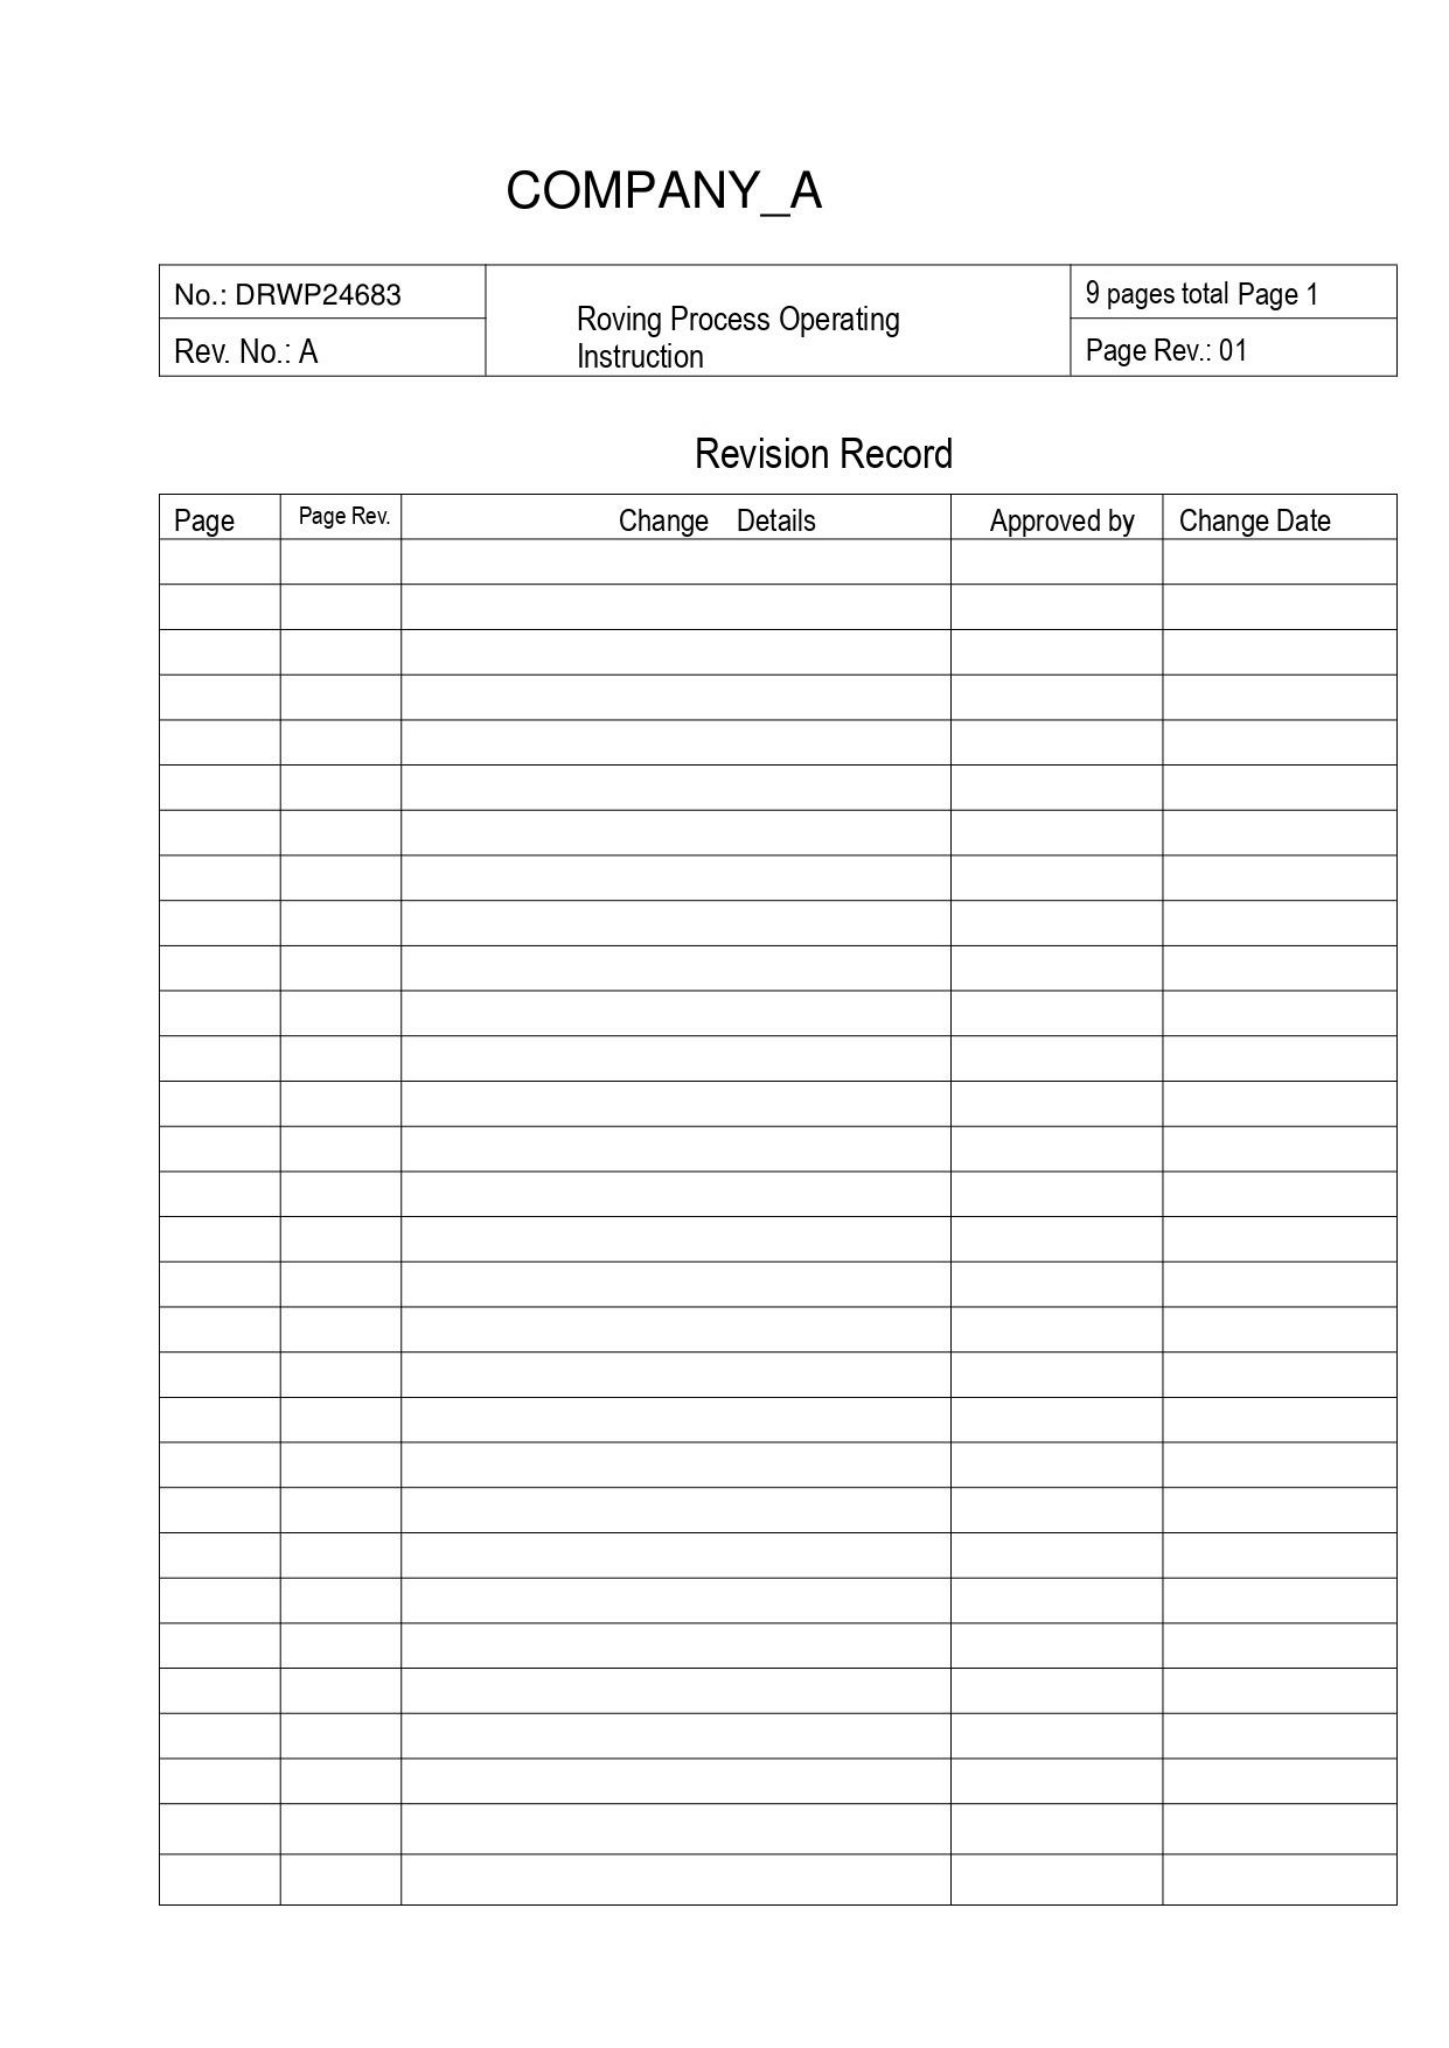COMPANY_A

| No.: DRWP24683 | Roving Process Operating Instruction | 9 pages total Page 1 |
|---|---|---|
| Rev. No.: A | | Page Rev.: 01 |

Revision Record

| Page | Page Rev. | Change Details | Approved by | Change Date |
|---|---|---|---|---|
| | | | | |
| | | | | |
| | | | | |
| | | | | |
| | | | | |
| | | | | |
| | | | | |
| | | | | |
| | | | | |
| | | | | |
| | | | | |
| | | | | |
| | | | | |
| | | | | |
| | | | | |
| | | | | |
| | | | | |
| | | | | |
| | | | | |
| | | | | |
| | | | | |
| | | | | |
| | | | | |
| | | | | |
| | | | | |
| | | | | |
| | | | | |
| | | | | |
| | | | | |
| | | | | |
| | | | | |
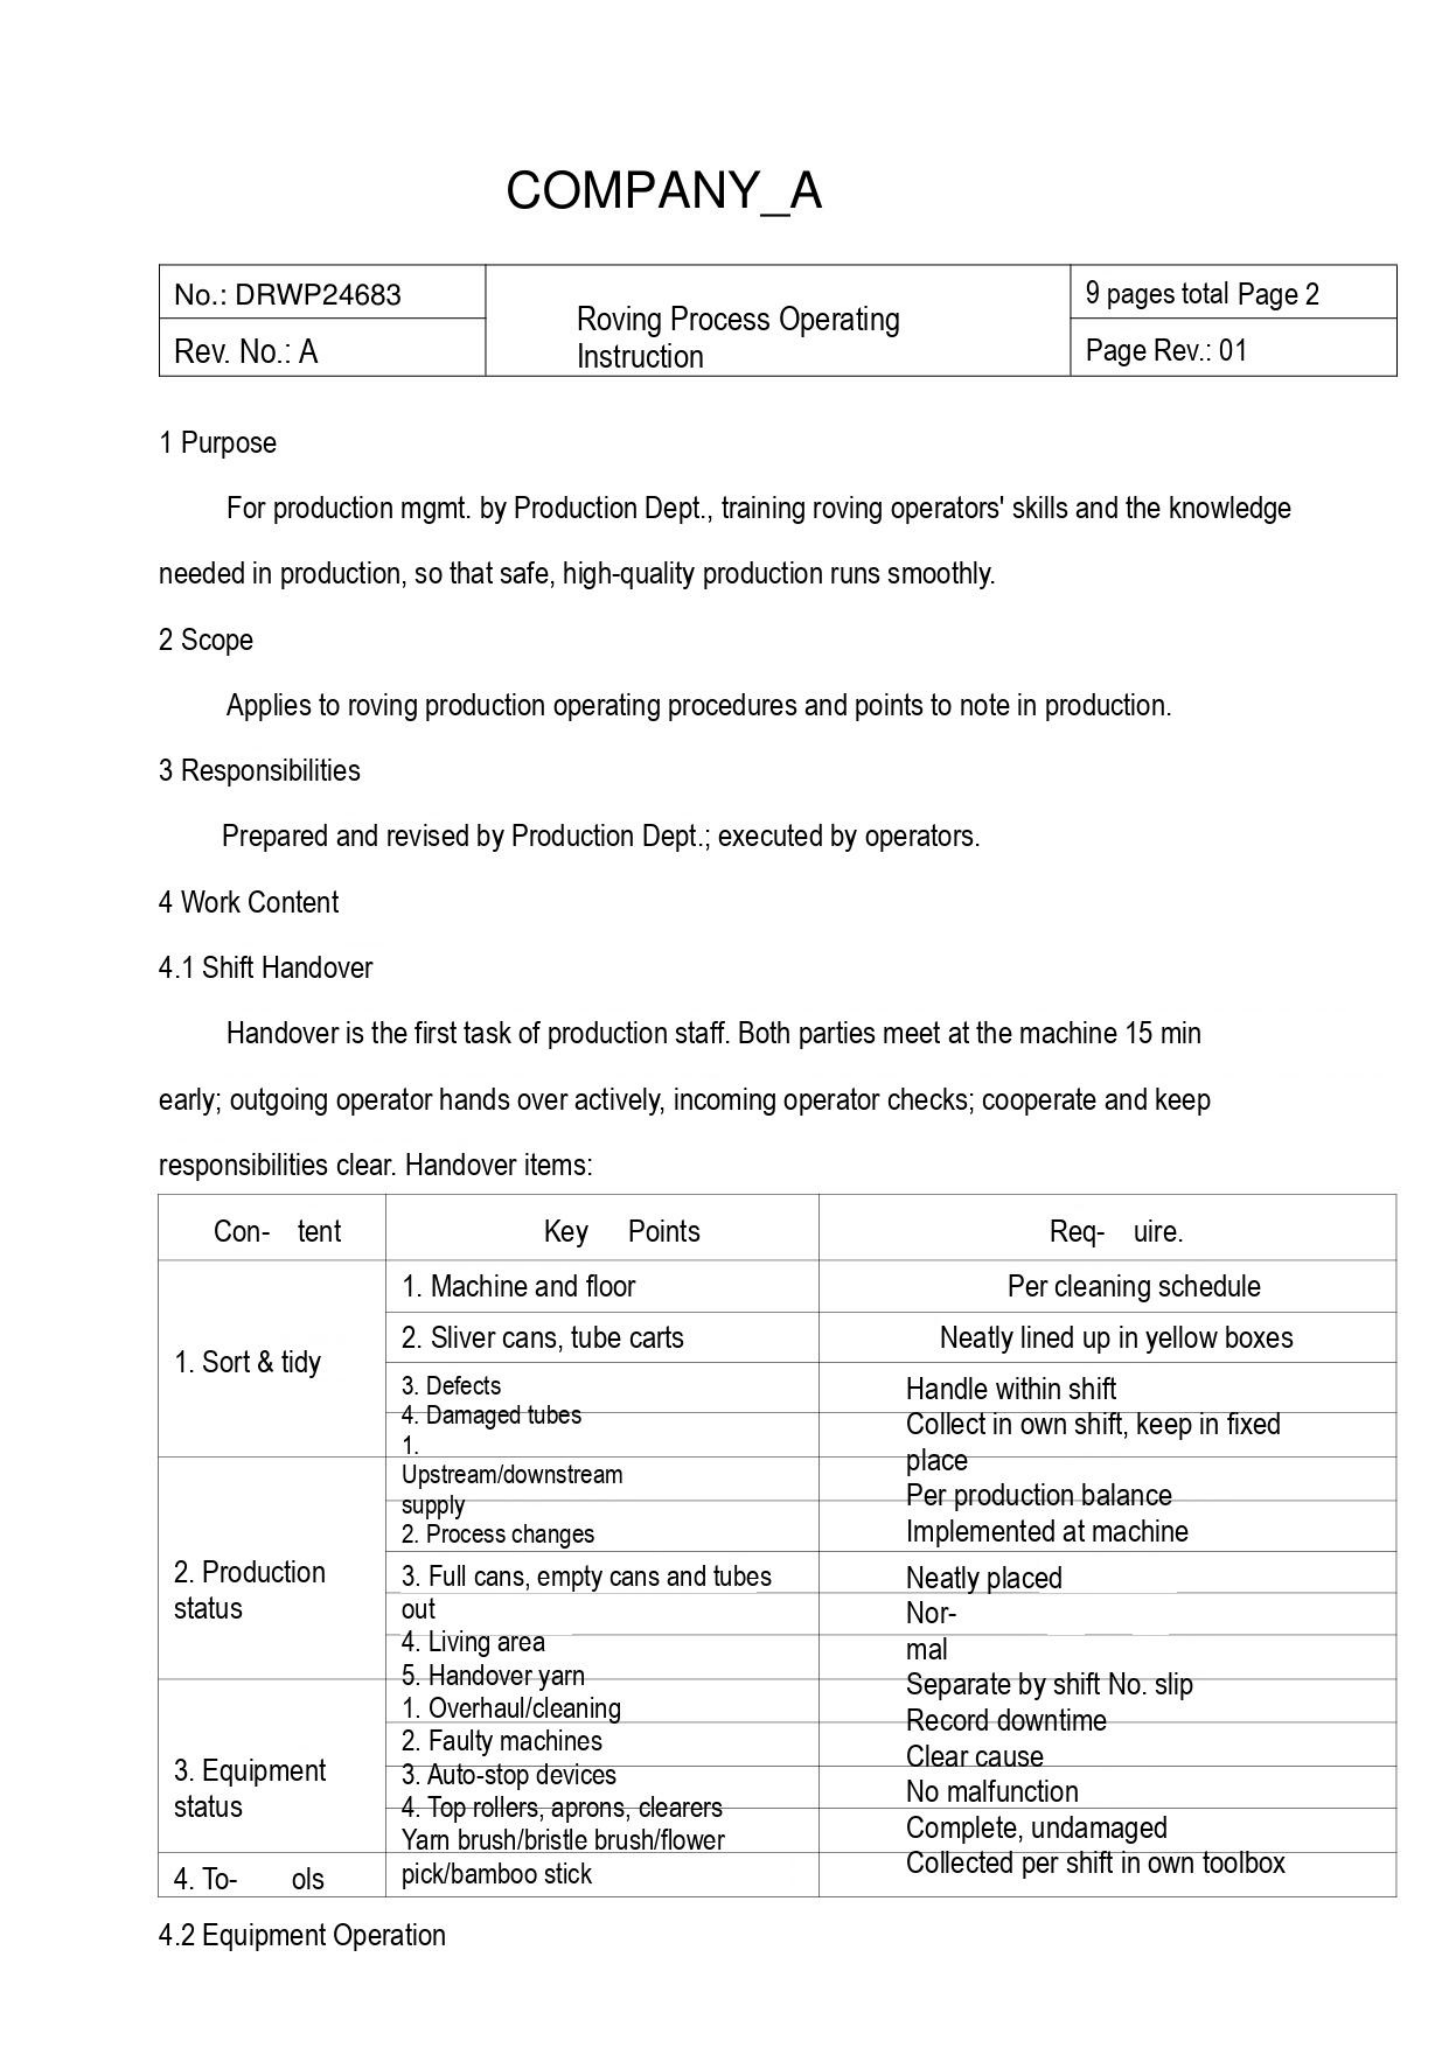# COMPANY_A

| No.: DRWP24683 | Roving Process Operating Instruction | 9 pages total Page 2 |
|---|---|---|
| Rev. No.: A | | Page Rev.: 01 |

1 Purpose

For production mgmt. by Production Dept., training roving operators' skills and the knowledge needed in production, so that safe, high-quality production runs smoothly.

2 Scope

Applies to roving production operating procedures and points to note in production.

3 Responsibilities

Prepared and revised by Production Dept.; executed by operators.

4 Work Content

4.1 Shift Handover

Handover is the first task of production staff. Both parties meet at the machine 15 min early; outgoing operator hands over actively, incoming operator checks; cooperate and keep responsibilities clear. Handover items:

| Con- tent | Key Points | Req- uire. |
|---|---|---|
| 1. Sort & tidy | 1. Machine and floor | Per cleaning schedule |
| | 2. Sliver cans, tube carts | Neatly lined up in yellow boxes |
| | 3. Defects | Handle within shift |
| | 4. Damaged tubes | Collect in own shift, keep in fixed place |
| 2. Production status | 1. Upstream/downstream supply | Per production balance |
| | 2. Process changes | Implemented at machine |
| | 3. Full cans, empty cans and tubes out | Neatly placed |
| | 4. Living area | Nor- mal |
| | 5. Handover yarn | Separate by shift No. slip |
| 3. Equipment status | 1. Overhaul/cleaning | Record downtime |
| | 2. Faulty machines | Clear cause |
| | 3. Auto-stop devices | No malfunction |
| | 4. Top rollers, aprons, clearers | Complete, undamaged |
| 4. To- ols | Yarn brush/bristle brush/flower pick/bamboo stick | Collected per shift in own toolbox |

4.2 Equipment Operation
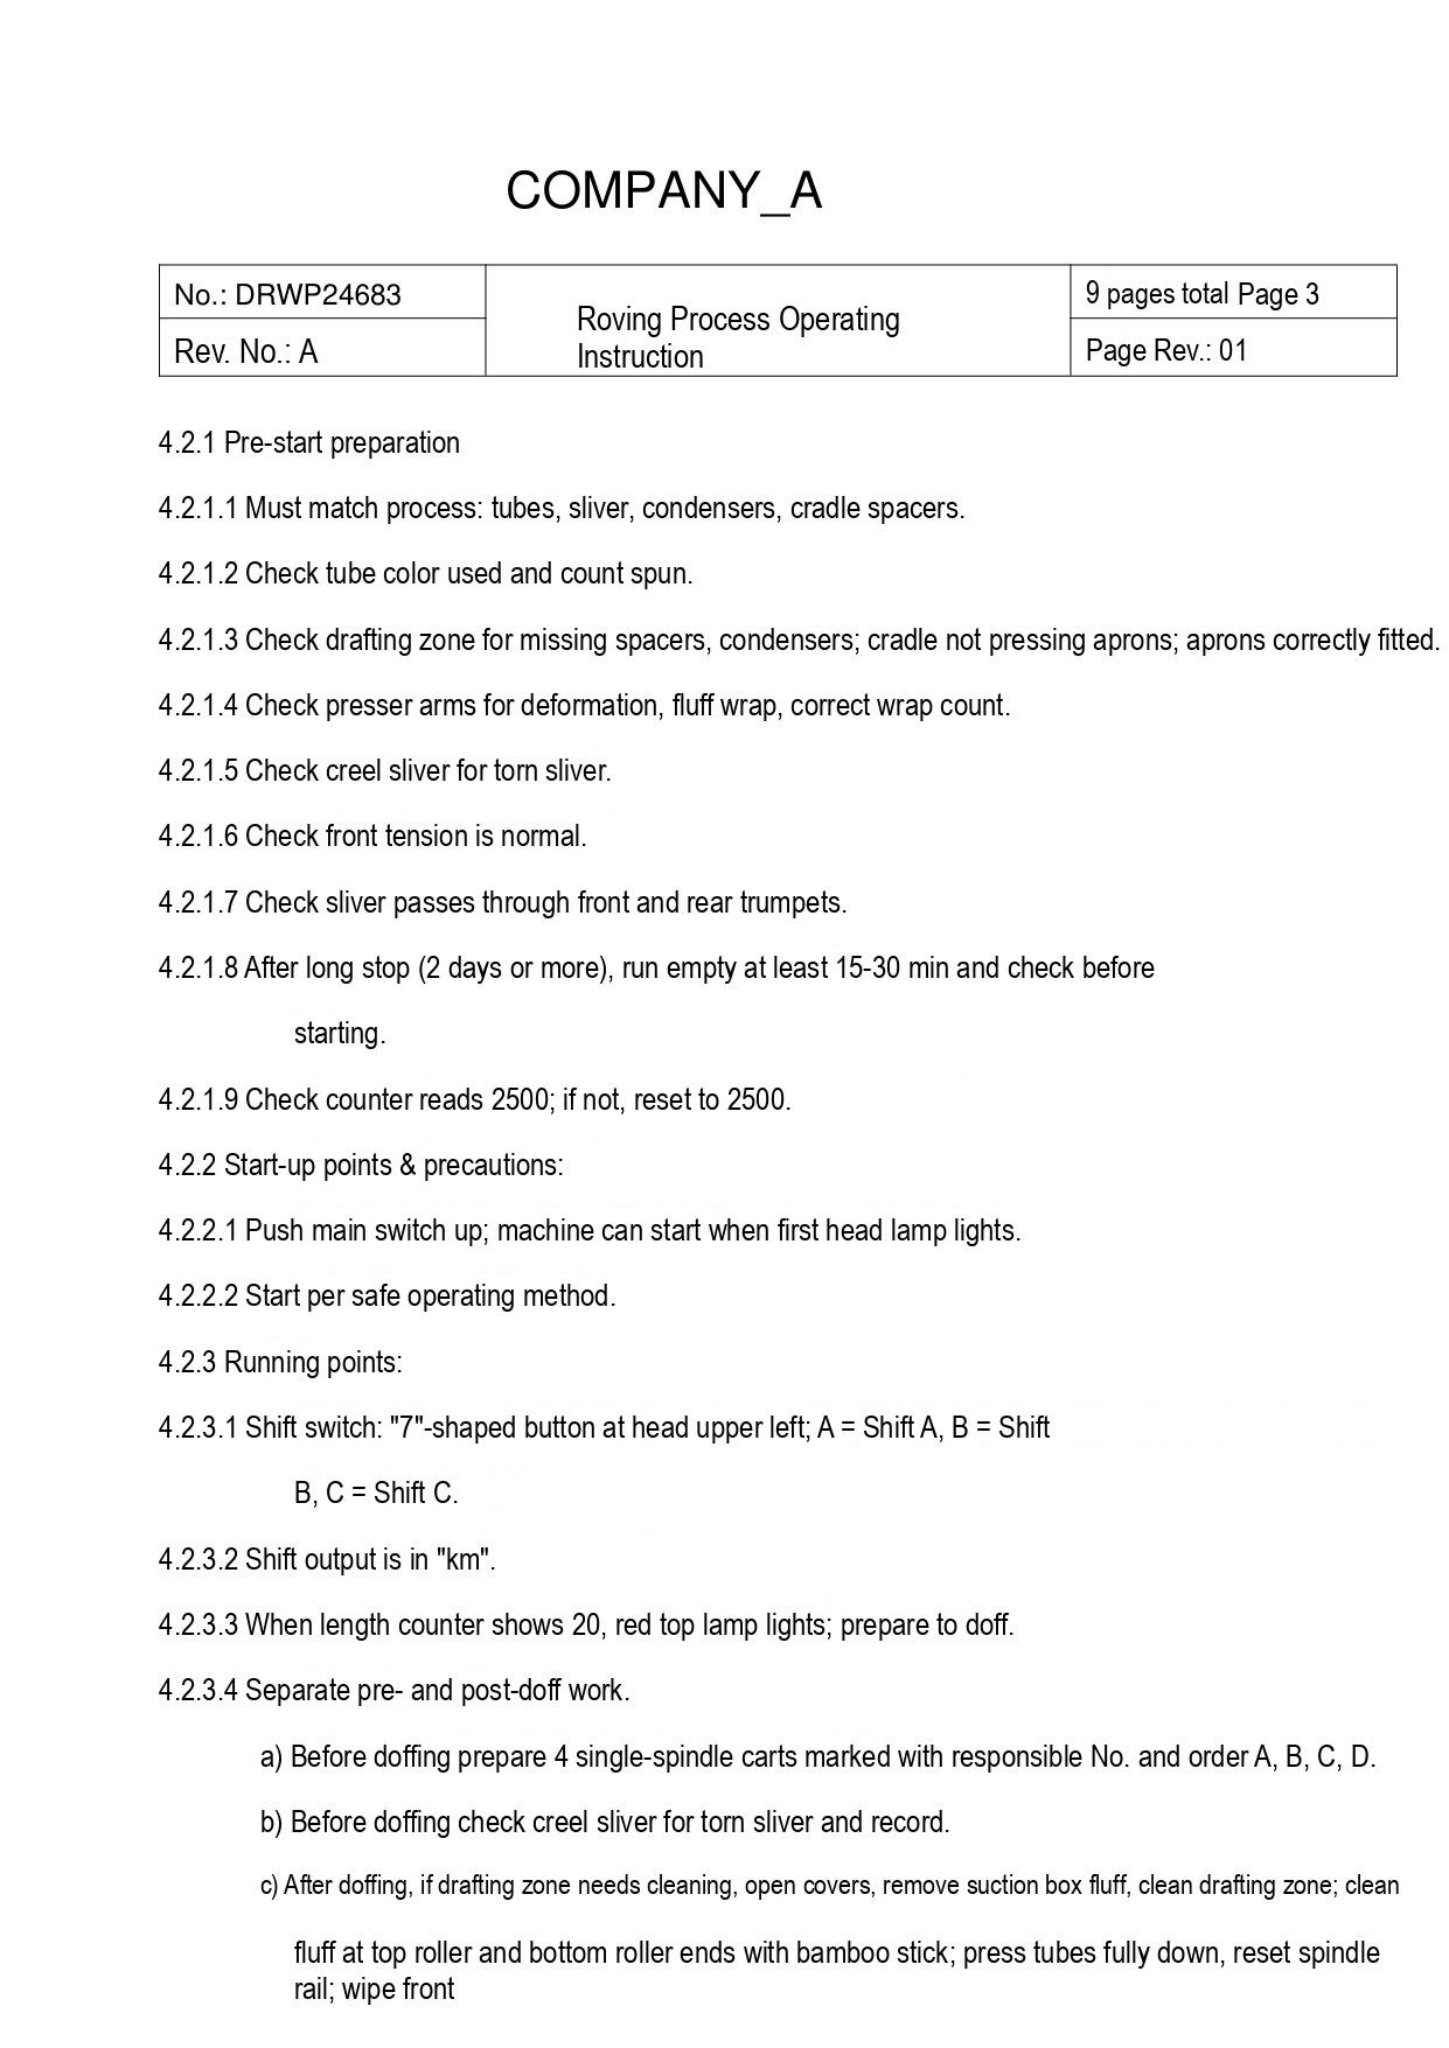COMPANY_A

| No.: DRWP24683 | Roving Process Operating Instruction | 9 pages total Page 3 |
|---|---|---|
| Rev. No.: A | | Page Rev.: 01 |

4.2.1 Pre-start preparation

4.2.1.1 Must match process: tubes, sliver, condensers, cradle spacers.

4.2.1.2 Check tube color used and count spun.

4.2.1.3 Check drafting zone for missing spacers, condensers; cradle not pressing aprons; aprons correctly fitted.

4.2.1.4 Check presser arms for deformation, fluff wrap, correct wrap count.

4.2.1.5 Check creel sliver for torn sliver.

4.2.1.6 Check front tension is normal.

4.2.1.7 Check sliver passes through front and rear trumpets.

4.2.1.8 After long stop (2 days or more), run empty at least 15-30 min and check before starting.

4.2.1.9 Check counter reads 2500; if not, reset to 2500.

4.2.2 Start-up points & precautions:

4.2.2.1 Push main switch up; machine can start when first head lamp lights.

4.2.2.2 Start per safe operating method.

4.2.3 Running points:

4.2.3.1 Shift switch: "7"-shaped button at head upper left; A = Shift A, B = Shift B, C = Shift C.

4.2.3.2 Shift output is in "km".

4.2.3.3 When length counter shows 20, red top lamp lights; prepare to doff.

4.2.3.4 Separate pre- and post-doff work.

a) Before doffing prepare 4 single-spindle carts marked with responsible No. and order A, B, C, D.

b) Before doffing check creel sliver for torn sliver and record.

c) After doffing, if drafting zone needs cleaning, open covers, remove suction box fluff, clean drafting zone; clean fluff at top roller and bottom roller ends with bamboo stick; press tubes fully down, reset spindle rail; wipe front
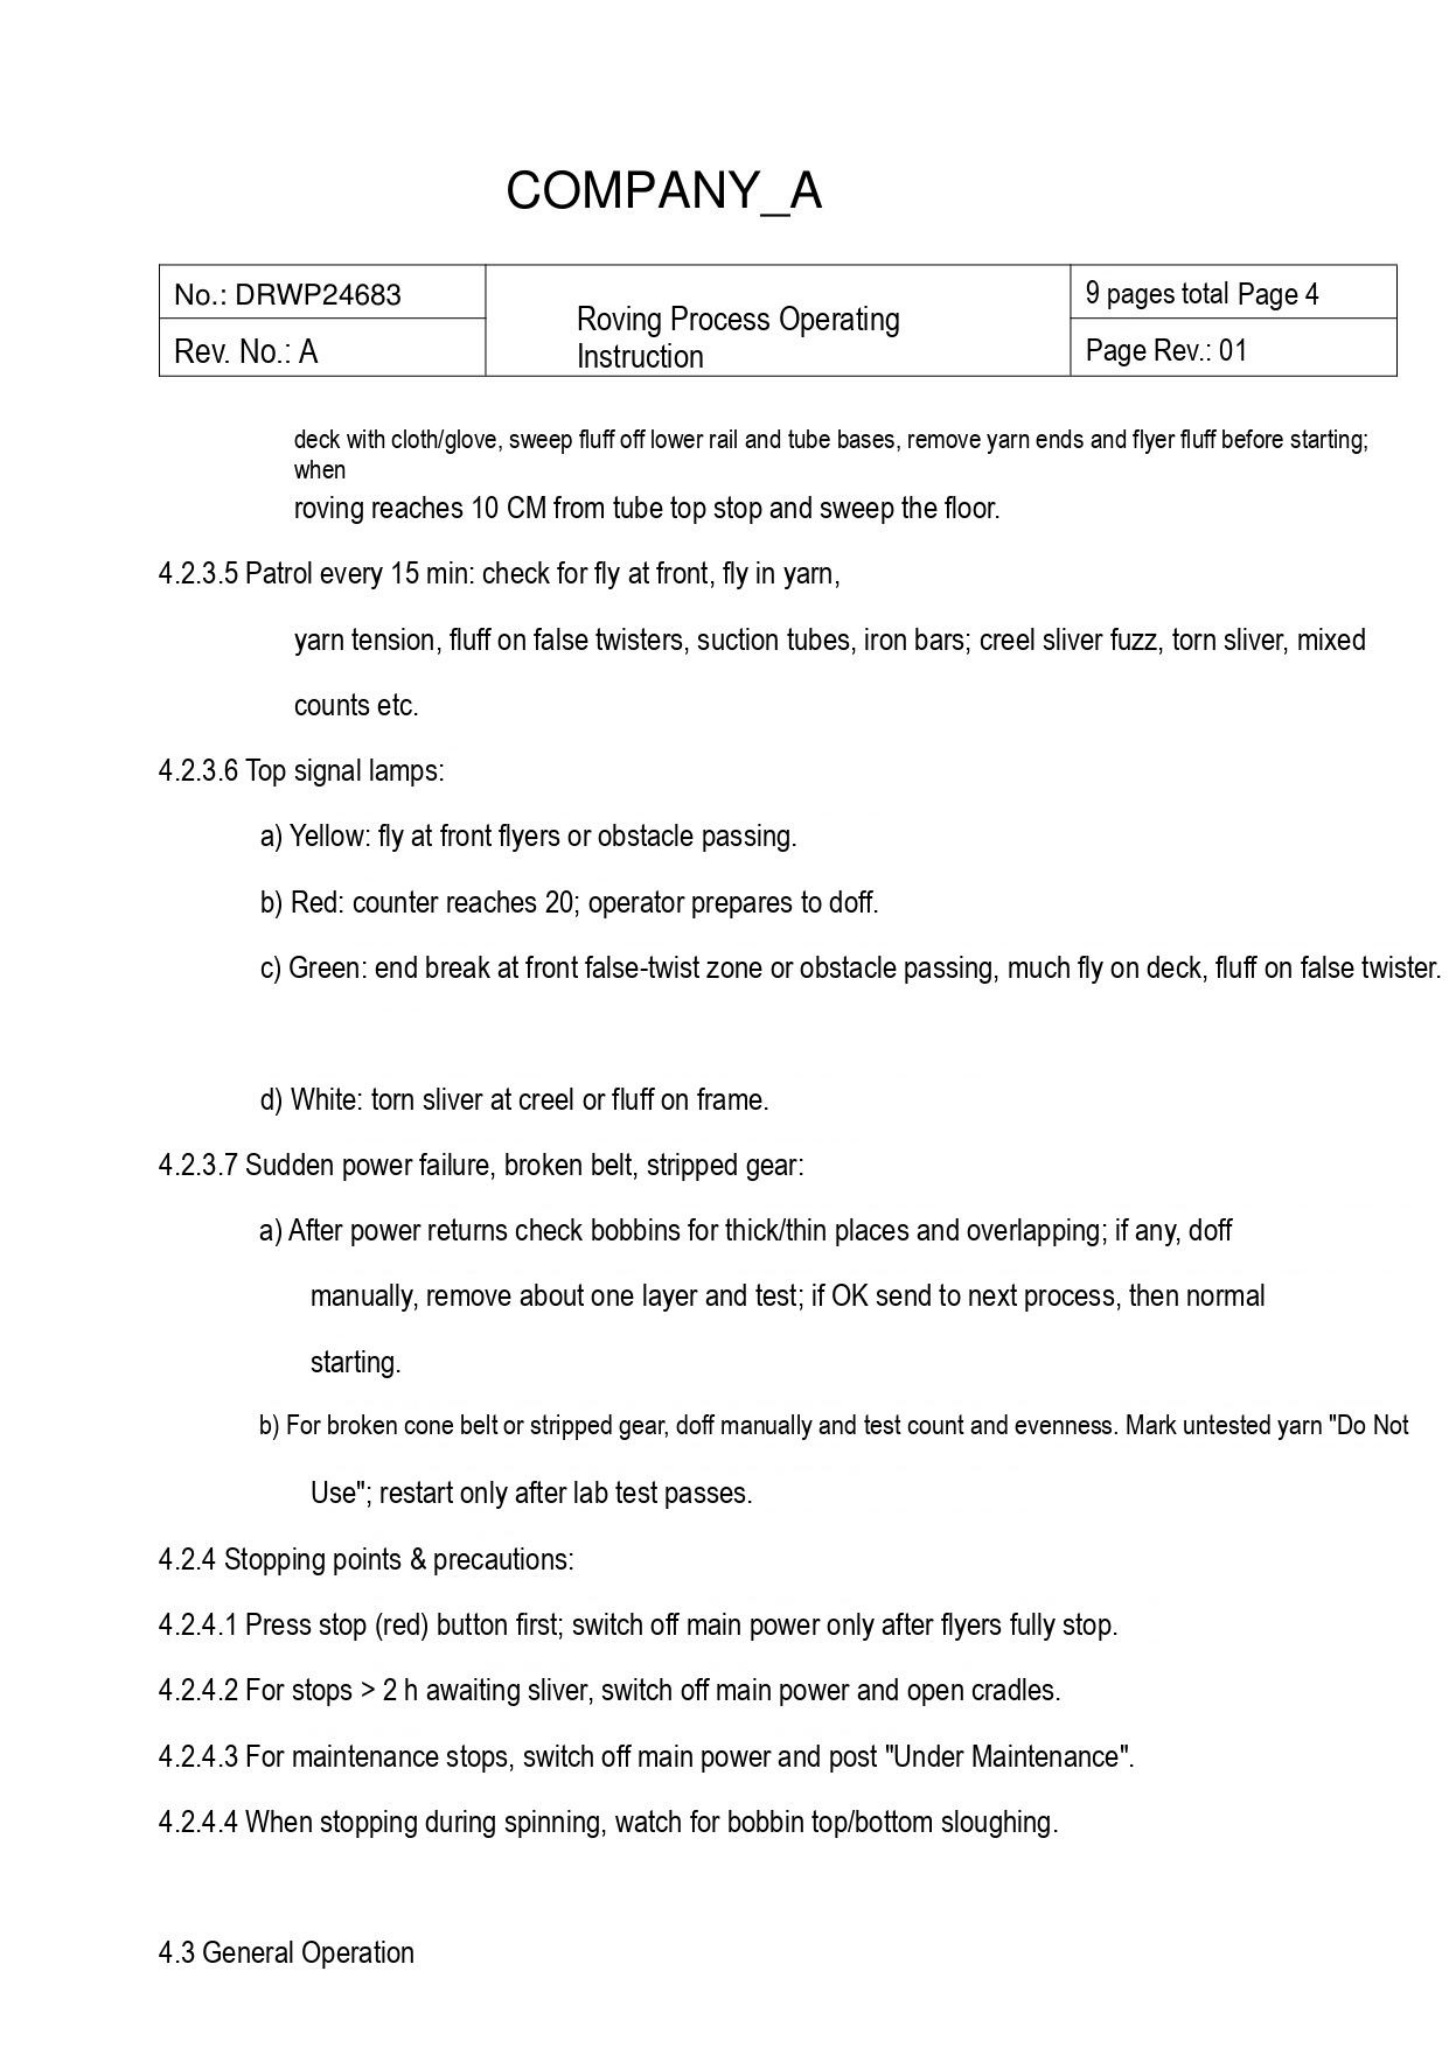COMPANY_A

| No.: DRWP24683 | Roving Process Operating Instruction | 9 pages total Page 4 |
|---|---|---|
| Rev. No.: A | | Page Rev.: 01 |

deck with cloth/glove, sweep fluff off lower rail and tube bases, remove yarn ends and flyer fluff before starting; when
roving reaches 10 CM from tube top stop and sweep the floor.

4.2.3.5 Patrol every 15 min: check for fly at front, fly in yarn,
yarn tension, fluff on false twisters, suction tubes, iron bars; creel sliver fuzz, torn sliver, mixed counts etc.

4.2.3.6 Top signal lamps:

a) Yellow: fly at front flyers or obstacle passing.

b) Red: counter reaches 20; operator prepares to doff.

c) Green: end break at front false-twist zone or obstacle passing, much fly on deck, fluff on false twister.

d) White: torn sliver at creel or fluff on frame.

4.2.3.7 Sudden power failure, broken belt, stripped gear:

a) After power returns check bobbins for thick/thin places and overlapping; if any, doff manually, remove about one layer and test; if OK send to next process, then normal starting.

b) For broken cone belt or stripped gear, doff manually and test count and evenness. Mark untested yarn "Do Not Use"; restart only after lab test passes.

4.2.4 Stopping points & precautions:

4.2.4.1 Press stop (red) button first; switch off main power only after flyers fully stop.

4.2.4.2 For stops > 2 h awaiting sliver, switch off main power and open cradles.

4.2.4.3 For maintenance stops, switch off main power and post "Under Maintenance".

4.2.4.4 When stopping during spinning, watch for bobbin top/bottom sloughing.

4.3 General Operation
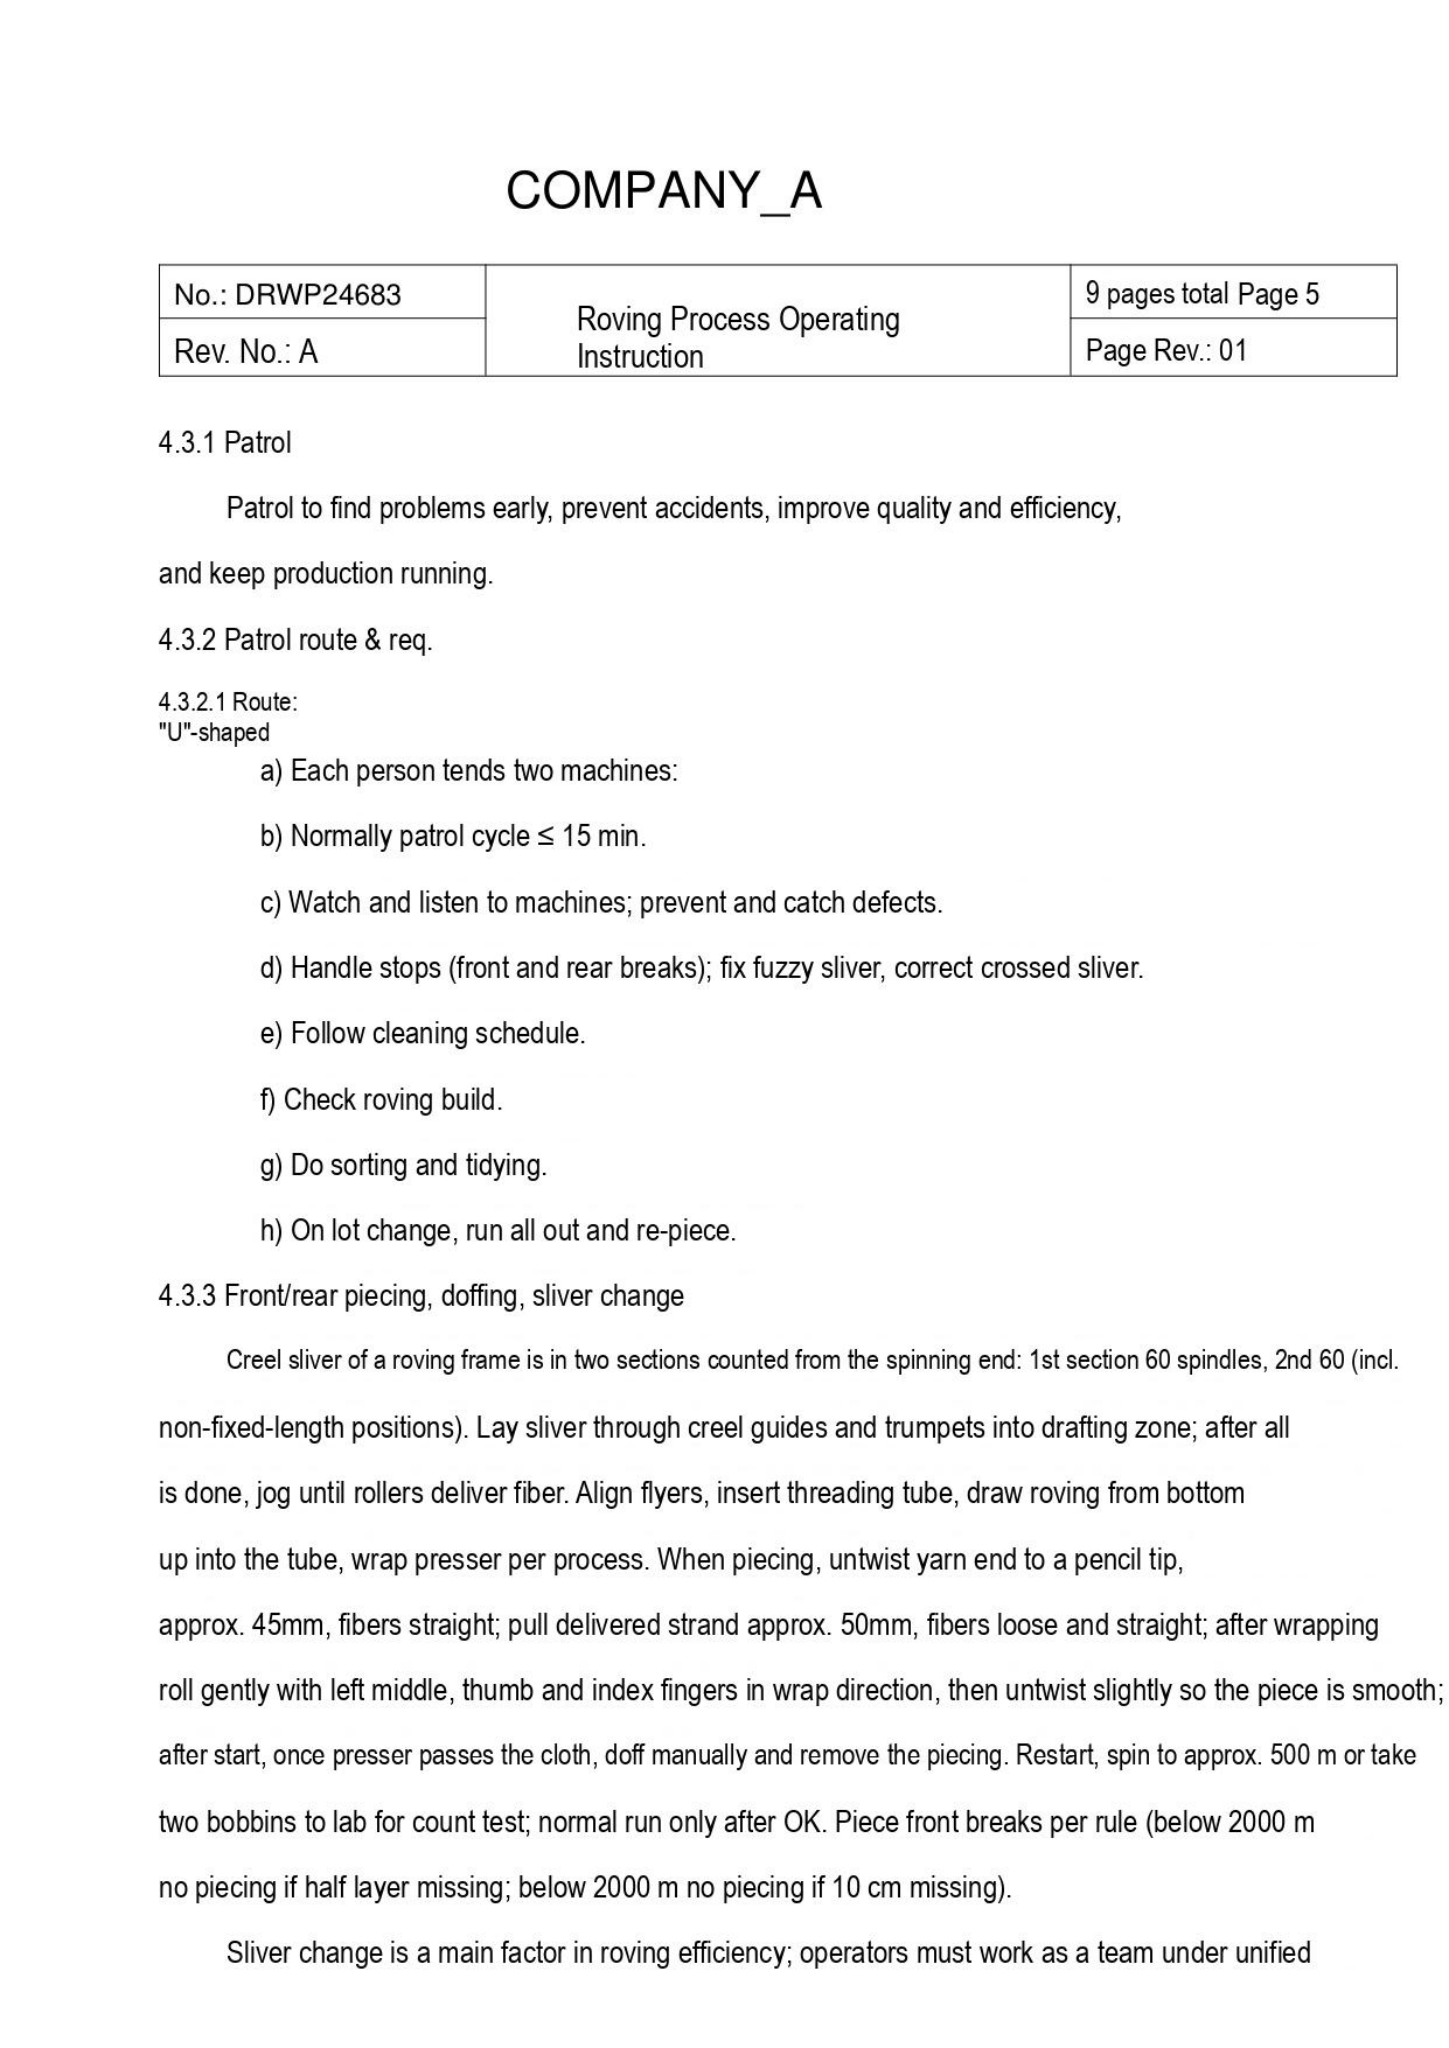COMPANY_A

| No.: DRWP24683 | Roving Process Operating Instruction | 9 pages total Page 5 |
|---|---|---|
| Rev. No.: A | | Page Rev.: 01 |

4.3.1 Patrol

Patrol to find problems early, prevent accidents, improve quality and efficiency, and keep production running.

4.3.2 Patrol route & req.

4.3.2.1 Route:
"U"-shaped

a) Each person tends two machines:

b) Normally patrol cycle ≤ 15 min.

c) Watch and listen to machines; prevent and catch defects.

d) Handle stops (front and rear breaks); fix fuzzy sliver, correct crossed sliver.

e) Follow cleaning schedule.

f) Check roving build.

g) Do sorting and tidying.

h) On lot change, run all out and re-piece.

4.3.3 Front/rear piecing, doffing, sliver change

Creel sliver of a roving frame is in two sections counted from the spinning end: 1st section 60 spindles, 2nd 60 (incl. non-fixed-length positions). Lay sliver through creel guides and trumpets into drafting zone; after all is done, jog until rollers deliver fiber. Align flyers, insert threading tube, draw roving from bottom up into the tube, wrap presser per process. When piecing, untwist yarn end to a pencil tip, approx. 45mm, fibers straight; pull delivered strand approx. 50mm, fibers loose and straight; after wrapping roll gently with left middle, thumb and index fingers in wrap direction, then untwist slightly so the piece is smooth; after start, once presser passes the cloth, doff manually and remove the piecing. Restart, spin to approx. 500 m or take two bobbins to lab for count test; normal run only after OK. Piece front breaks per rule (below 2000 m no piecing if half layer missing; below 2000 m no piecing if 10 cm missing).

Sliver change is a main factor in roving efficiency; operators must work as a team under unified
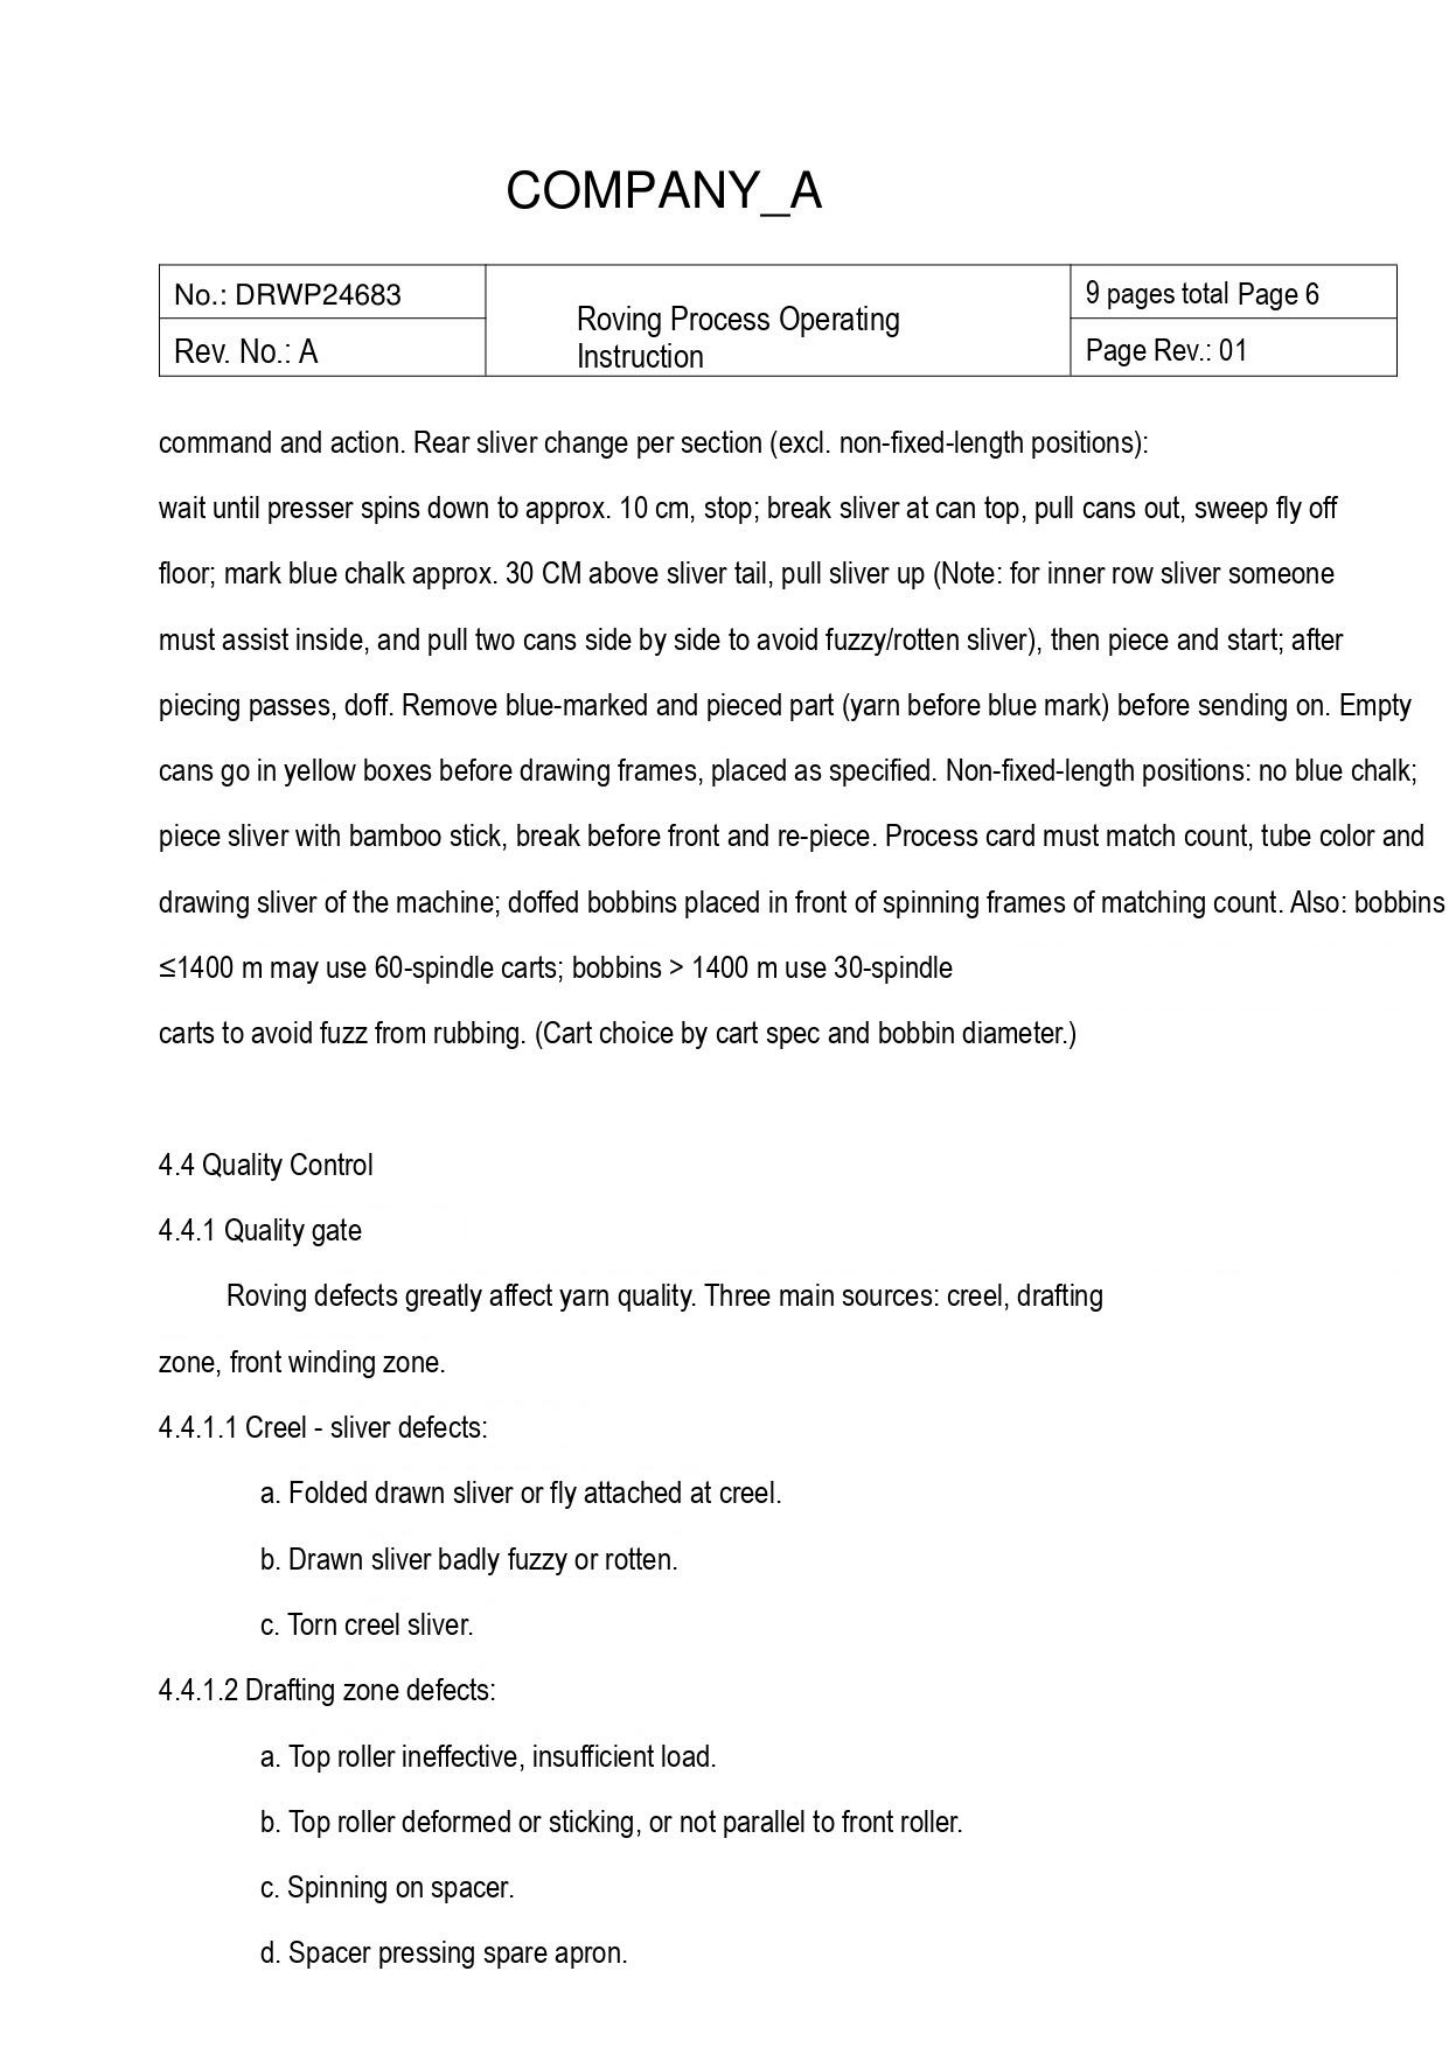COMPANY_A

| No.: DRWP24683 | Roving Process Operating Instruction | 9 pages total Page 6 |
|---|---|---|
| Rev. No.: A | | Page Rev.: 01 |

command and action. Rear sliver change per section (excl. non-fixed-length positions): wait until presser spins down to approx. 10 cm, stop; break sliver at can top, pull cans out, sweep fly off floor; mark blue chalk approx. 30 CM above sliver tail, pull sliver up (Note: for inner row sliver someone must assist inside, and pull two cans side by side to avoid fuzzy/rotten sliver), then piece and start; after piecing passes, doff. Remove blue-marked and pieced part (yarn before blue mark) before sending on. Empty cans go in yellow boxes before drawing frames, placed as specified. Non-fixed-length positions: no blue chalk; piece sliver with bamboo stick, break before front and re-piece. Process card must match count, tube color and drawing sliver of the machine; doffed bobbins placed in front of spinning frames of matching count. Also: bobbins ≤1400 m may use 60-spindle carts; bobbins > 1400 m use 30-spindle carts to avoid fuzz from rubbing. (Cart choice by cart spec and bobbin diameter.)

4.4 Quality Control

4.4.1 Quality gate

Roving defects greatly affect yarn quality. Three main sources: creel, drafting zone, front winding zone.

4.4.1.1 Creel - sliver defects:

a. Folded drawn sliver or fly attached at creel.

b. Drawn sliver badly fuzzy or rotten.

c. Torn creel sliver.

4.4.1.2 Drafting zone defects:

a. Top roller ineffective, insufficient load.

b. Top roller deformed or sticking, or not parallel to front roller.

c. Spinning on spacer.

d. Spacer pressing spare apron.
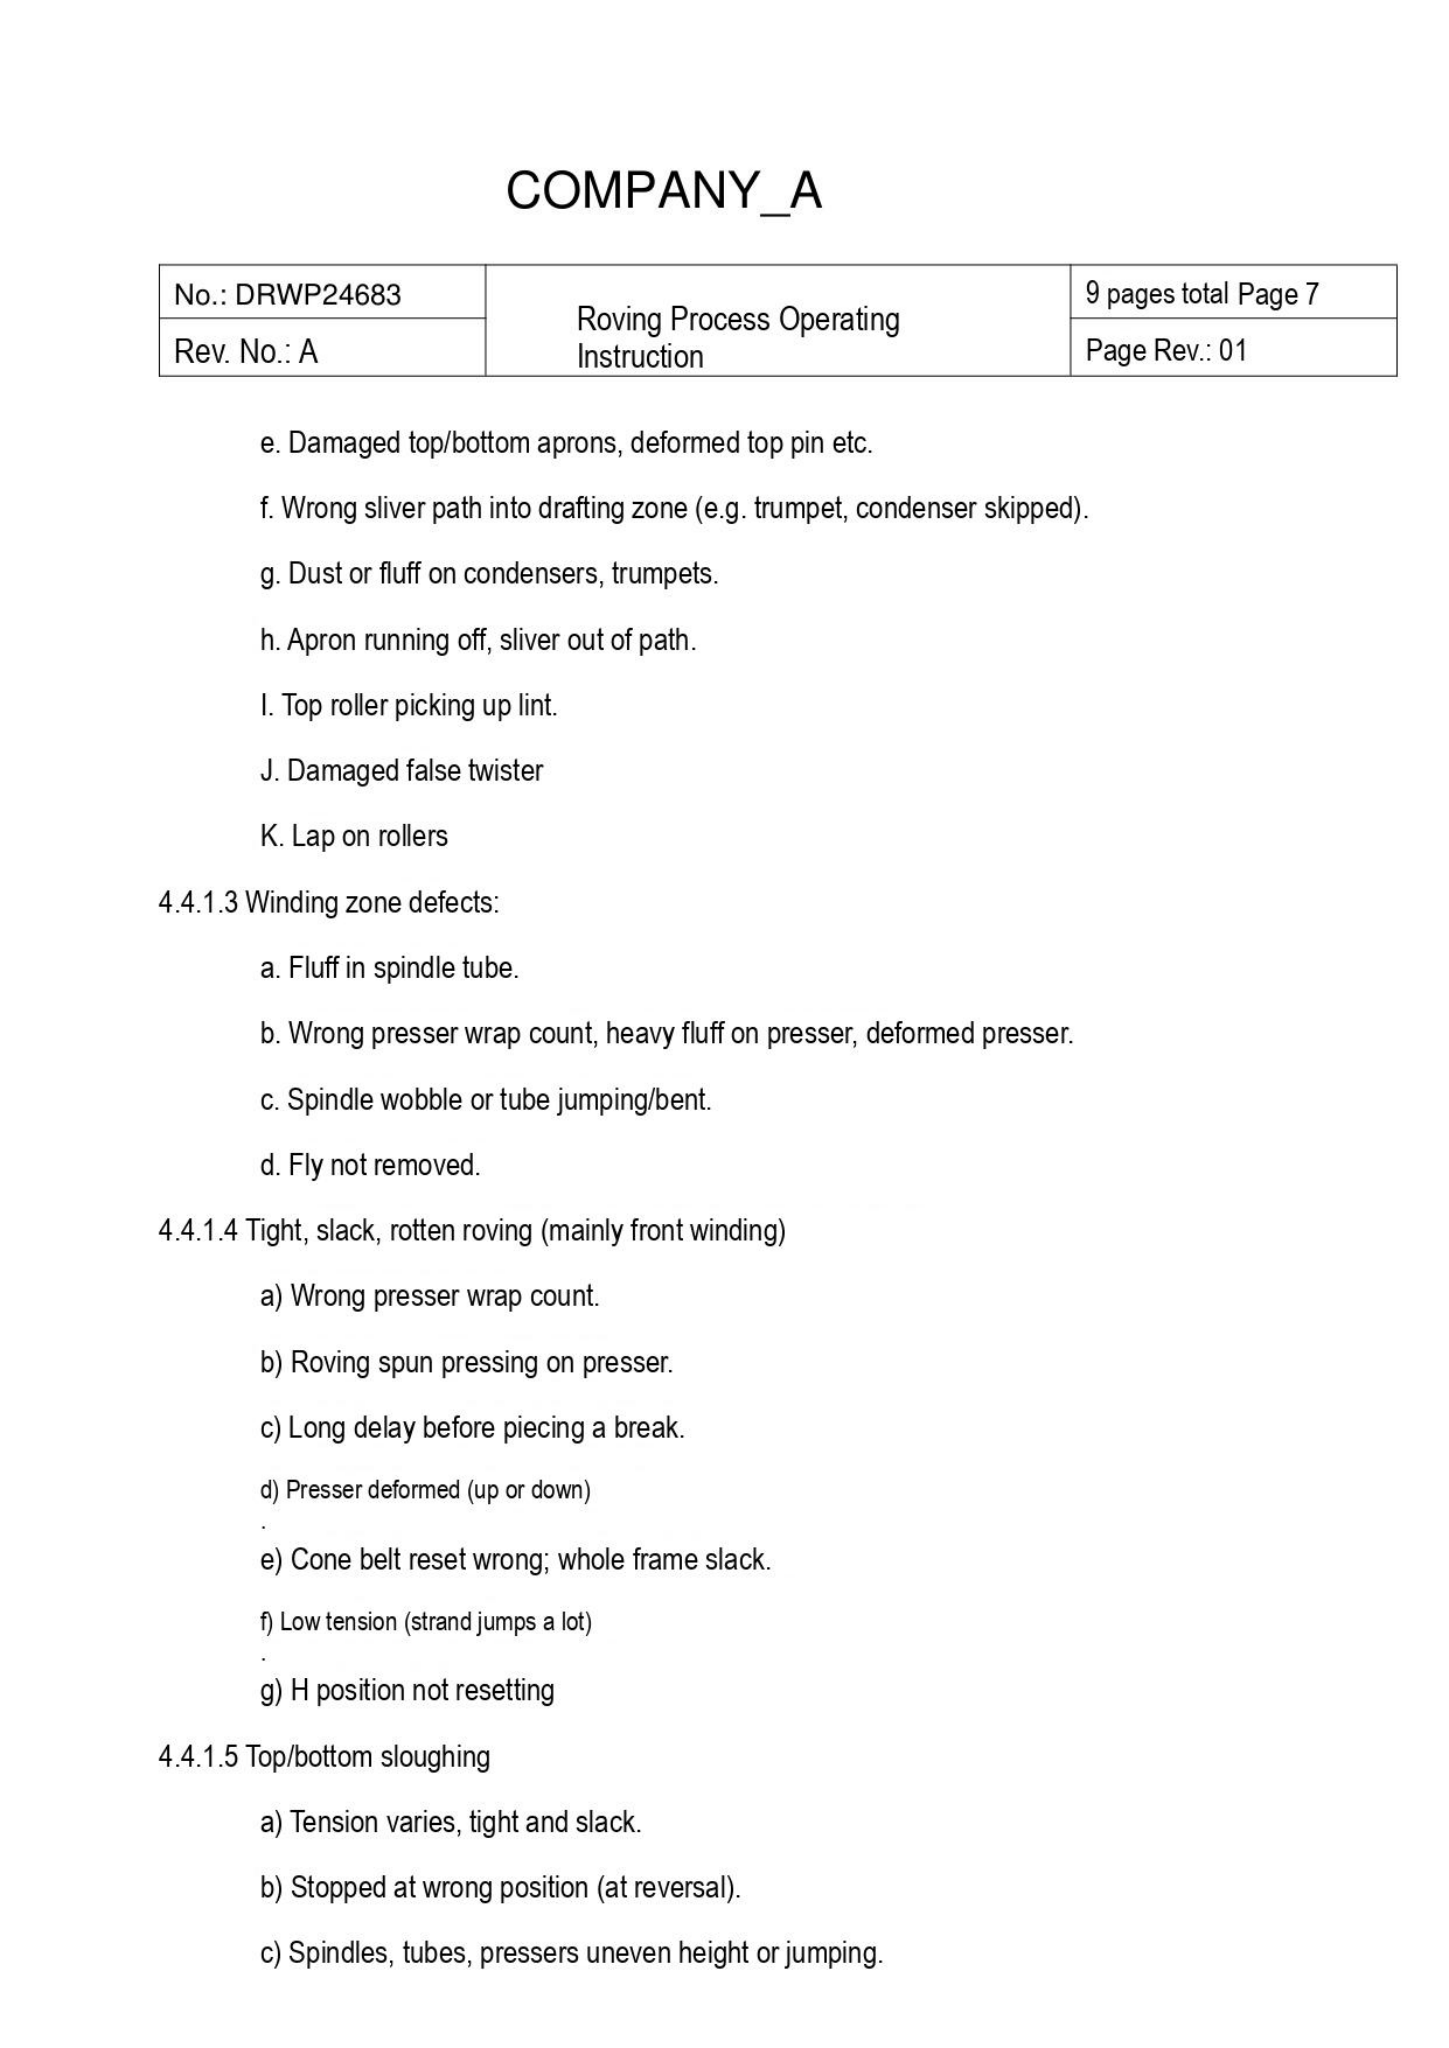COMPANY_A

| No.: DRWP24683 | Roving Process Operating Instruction | 9 pages total Page 7 |
|---|---|---|
| Rev. No.: A | | Page Rev.: 01 |

e. Damaged top/bottom aprons, deformed top pin etc.

f. Wrong sliver path into drafting zone (e.g. trumpet, condenser skipped).

g. Dust or fluff on condensers, trumpets.

h. Apron running off, sliver out of path.

I. Top roller picking up lint.

J. Damaged false twister

K. Lap on rollers

4.4.1.3 Winding zone defects:

a. Fluff in spindle tube.

b. Wrong presser wrap count, heavy fluff on presser, deformed presser.

c. Spindle wobble or tube jumping/bent.

d. Fly not removed.

4.4.1.4 Tight, slack, rotten roving (mainly front winding)

a) Wrong presser wrap count.

b) Roving spun pressing on presser.

c) Long delay before piecing a break.

d) Presser deformed (up or down)

e) Cone belt reset wrong; whole frame slack.

f) Low tension (strand jumps a lot)

g) H position not resetting

4.4.1.5 Top/bottom sloughing

a) Tension varies, tight and slack.

b) Stopped at wrong position (at reversal).

c) Spindles, tubes, pressers uneven height or jumping.